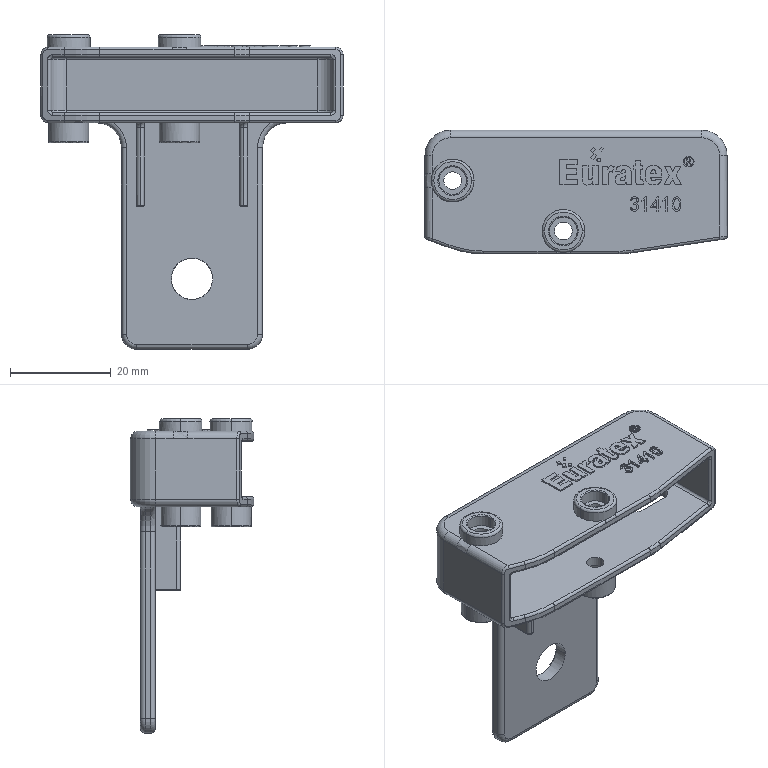Part | STEP file | 101000007605 | 1 solid | 364 faces | box 60 x 24.5 x 62.5 mm | volume 11628 mm3 | plane 180 | cylinder 96 | torus 48 | spline 38 | cone 2 | commonest cylinder face diameters 1 x23 3.5 x8 3 x7 2 x6 0.4 x4 0.6 x4